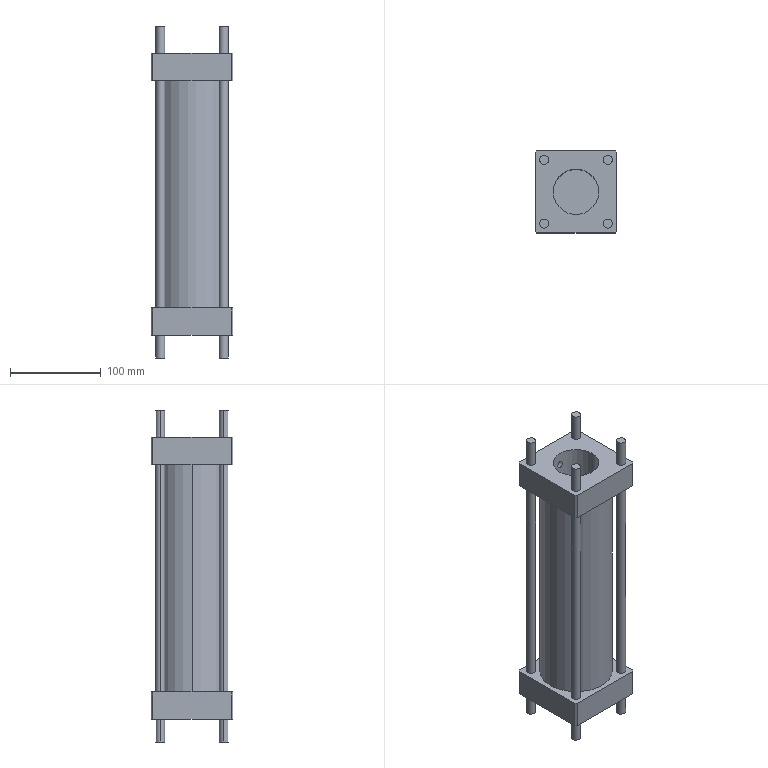Part | STEP file | Telescopic Hydraulic Cylinder | 1 solid | 71 faces | box 90 x 90 x 365 mm | volume 1281349 mm3 | cylinder 32 | plane 31 | cone 8 | commonest cylinder face diameters 10 x24 14.3 x4 50 x2 80 x2